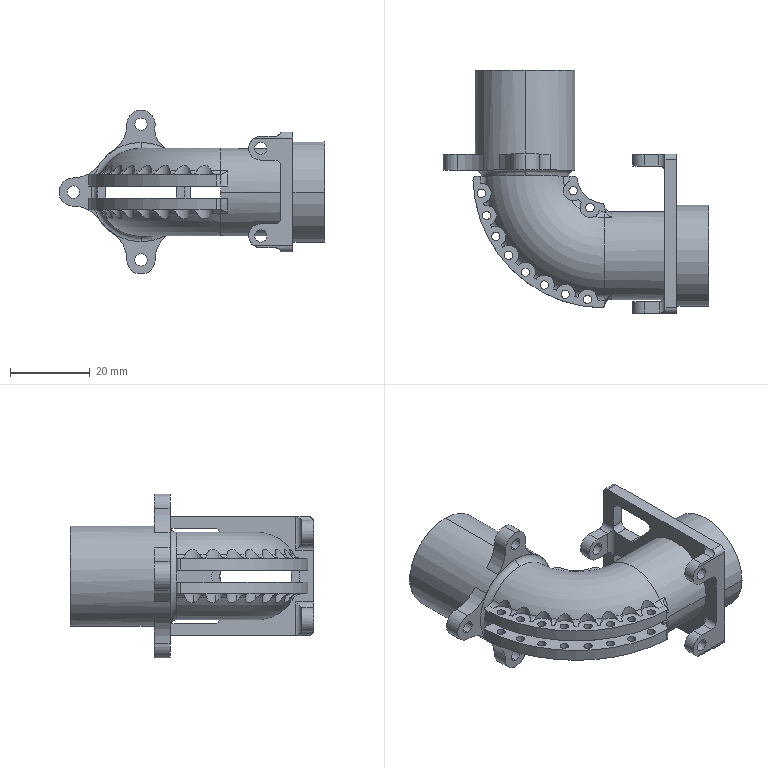Part | SolidWorks | features ICE 15, Fillet 6, Chamfer 2, Extrusion 1, MirrorPattern 1, RevCut 1, Revolution 1 | 1 solid | 245 faces | box 66.65 x 61 x 41.1 mm | volume 16016 mm3 | cylinder 150 | plane 51 | torus 34 | cone 6 | spline 4 | commonest cylinder face diameters 2.1 x40 5 x30 3 x23 3.1 x12 2 x9 3.6 x4